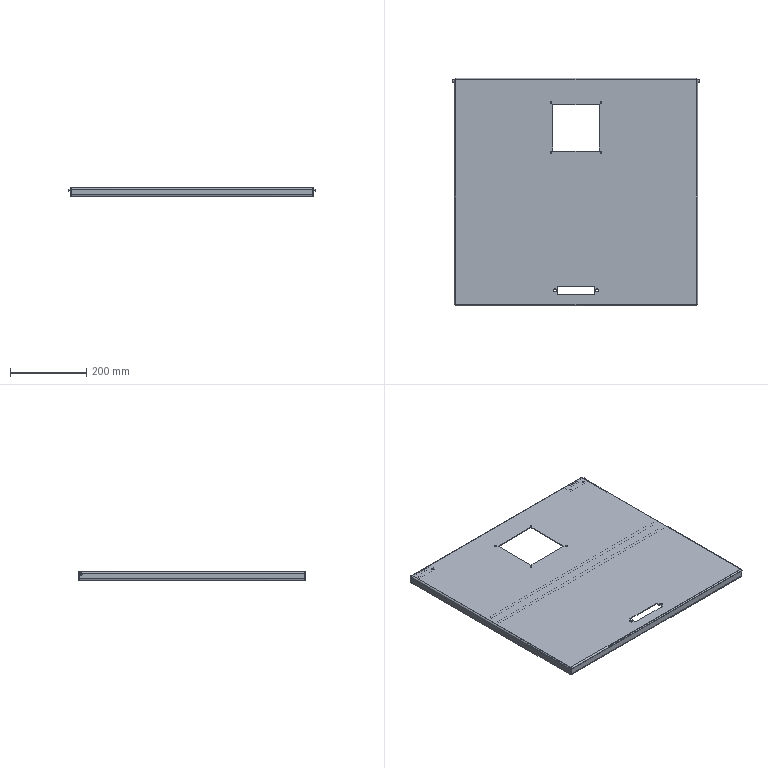Part | NX | features BREP 8 | 8 solids | 280 faces | box 648 x 597 x 23.5 mm | volume 953778 mm3 | plane 108 | cylinder 76 | torus 76 | spline 16 | cone 4 | commonest cylinder face diameters 6 x16 4 x12 8 x12 10 x12 5 x8 5.3 x8